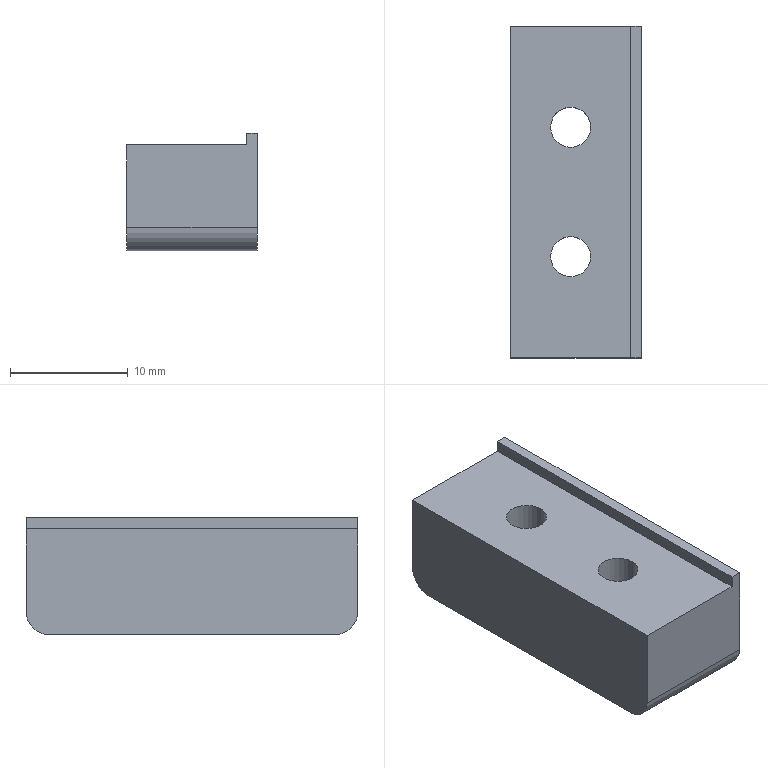Part | STEP file | 11-FG-SZ00911 | 1 solid | 20 faces | box 11.1 x 28.2 x 10 mm | volume 2496 mm3 | cylinder 10 | plane 10 | commonest cylinder face diameters 3.4 x4 6.5 x4 4 x2
STEP:
#1=CARTESIAN_POINT('',(3.25,5.5,3.4));
#2=VERTEX_POINT('',#1);
#3=CARTESIAN_POINT('',(-3.25,5.5,3.4));
#4=VERTEX_POINT('',#3);
#5=CARTESIAN_POINT('',(0.,5.5,3.4));
#6=DIRECTION('',(0.,0.,-1.));
#7=DIRECTION('',(-1.,0.,0.));
#8=AXIS2_PLACEMENT_3D('',#5,#6,#7);
#9=CIRCLE('',#8,3.25);
#10=EDGE_CURVE('',#2,#4,#9,.T.);
#11=ORIENTED_EDGE('',*,*,#10,.F.);
#12=CARTESIAN_POINT('',(3.25,5.5,0.));
#13=VERTEX_POINT('',#12);
#14=CARTESIAN_POINT('',(3.25,5.5,0.));
#15=DIRECTION('',(0.,0.,-1.));
#16=VECTOR('',#15,1000.);
#17=LINE('',#14,#16);
#18=EDGE_CURVE('',#2,#13,#17,.T.);
#19=ORIENTED_EDGE('',*,*,#18,.T.);
#20=CARTESIAN_POINT('',(-3.25,5.5,0.));
#21=VERTEX_POINT('',#20);
#22=CARTESIAN_POINT('',(0.,5.5,0.));
#23=DIRECTION('',(0.,0.,-1.));
#24=DIRECTION('',(-1.,0.,0.));
#25=AXIS2_PLACEMENT_3D('',#22,#23,#24);
#26=CIRCLE('',#25,3.25);
#27=EDGE_CURVE('',#13,#21,#26,.T.);
#28=ORIENTED_EDGE('',*,*,#27,.T.);
#29=CARTESIAN_POINT('',(-3.25,5.5,0.));
#30=DIRECTION('',(0.,0.,-1.));
#31=VECTOR('',#30,1000.);
#32=LINE('',#29,#31);
#33=EDGE_CURVE('',#4,#21,#32,.T.);
#34=ORIENTED_EDGE('',*,*,#33,.F.);
#35=EDGE_LOOP('',(#11,#19,#28,#34));
#36=FACE_OUTER_BOUND('',#35,.T.);
#37=CARTESIAN_POINT('',(0.,5.5,0.));
#38=DIRECTION('',(0.,0.,-1.));
#39=DIRECTION('',(-1.,0.,0.));
#40=AXIS2_PLACEMENT_3D('',#37,#38,#39);
#41=CYLINDRICAL_SURFACE('',#40,3.25);
#42=ADVANCED_FACE('',(#36),#41,.F.);
#43=CARTESIAN_POINT('',(1.7,5.5,9.));
#44=VERTEX_POINT('',#43);
#45=CARTESIAN_POINT('',(-1.7,5.5,9.));
#46=VERTEX_POINT('',#45);
#47=CARTESIAN_POINT('',(0.,5.5,9.));
#48=DIRECTION('',(0.,0.,-1.));
#49=DIRECTION('',(-1.,0.,0.));
#50=AXIS2_PLACEMENT_3D('',#47,#48,#49);
#51=CIRCLE('',#50,1.7);
#52=EDGE_CURVE('',#44,#46,#51,.T.);
#53=ORIENTED_EDGE('',*,*,#52,.F.);
#54=CARTESIAN_POINT('',(1.7,5.5,3.4));
#55=VERTEX_POINT('',#54);
#56=CARTESIAN_POINT('',(1.7,5.5,0.));
#57=DIRECTION('',(0.,0.,-1.));
#58=VECTOR('',#57,1000.);
#59=LINE('',#56,#58);
#60=EDGE_CURVE('',#44,#55,#59,.T.);
#61=ORIENTED_EDGE('',*,*,#60,.T.);
#62=CARTESIAN_POINT('',(-1.7,5.5,3.4));
#63=VERTEX_POINT('',#62);
#64=CARTESIAN_POINT('',(0.,5.5,3.4));
#65=DIRECTION('',(0.,0.,-1.));
#66=DIRECTION('',(-1.,0.,0.));
#67=AXIS2_PLACEMENT_3D('',#64,#65,#66);
#68=CIRCLE('',#67,1.7);
#69=EDGE_CURVE('',#55,#63,#68,.T.);
#70=ORIENTED_EDGE('',*,*,#69,.T.);
#71=CARTESIAN_POINT('',(-1.7,5.5,0.));
#72=DIRECTION('',(0.,0.,-1.));
#73=VECTOR('',#72,1000.);
#74=LINE('',#71,#73);
#75=EDGE_CURVE('',#46,#63,#74,.T.);
#76=ORIENTED_EDGE('',*,*,#75,.F.);
#77=EDGE_LOOP('',(#53,#61,#70,#76));
#78=FACE_OUTER_BOUND('',#77,.T.);
#79=CARTESIAN_POINT('',(0.,5.5,0.));
#80=DIRECTION('',(0.,0.,-1.));
#81=DIRECTION('',(-1.,0.,0.));
#82=AXIS2_PLACEMENT_3D('',#79,#80,#81);
#83=CYLINDRICAL_SURFACE('',#82,1.7);
#84=ADVANCED_FACE('',(#78),#83,.F.);
#85=CARTESIAN_POINT('',(3.25,-5.5,3.4));
#86=VERTEX_POINT('',#85);
#87=CARTESIAN_POINT('',(-3.25,-5.5,3.4));
#88=VERTEX_POINT('',#87);
#89=CARTESIAN_POINT('',(0.,-5.5,3.4));
#90=DIRECTION('',(0.,0.,-1.));
#91=DIRECTION('',(-1.,0.,0.));
#92=AXIS2_PLACEMENT_3D('',#89,#90,#91);
#93=CIRCLE('',#92,3.25);
#94=EDGE_CURVE('',#86,#88,#93,.T.);
#95=ORIENTED_EDGE('',*,*,#94,.F.);
#96=CARTESIAN_POINT('',(3.25,-5.5,0.));
#97=VERTEX_POINT('',#96);
#98=CARTESIAN_POINT('',(3.25,-5.5,0.));
#99=DIRECTION('',(0.,0.,-1.));
#100=VECTOR('',#99,1000.);
#101=LINE('',#98,#100);
#102=EDGE_CURVE('',#86,#97,#101,.T.);
#103=ORIENTED_EDGE('',*,*,#102,.T.);
#104=CARTESIAN_POINT('',(-3.25,-5.5,0.));
#105=VERTEX_POINT('',#104);
#106=CARTESIAN_POINT('',(0.,-5.5,0.));
#107=DIRECTION('',(0.,0.,-1.));
#108=DIRECTION('',(-1.,0.,0.));
#109=AXIS2_PLACEMENT_3D('',#106,#107,#108);
#110=CIRCLE('',#109,3.25);
#111=EDGE_CURVE('',#97,#105,#110,.T.);
#112=ORIENTED_EDGE('',*,*,#111,.T.);
#113=CARTESIAN_POINT('',(-3.25,-5.5,0.));
#114=DIRECTION('',(0.,0.,-1.));
#115=VECTOR('',#114,1000.);
#116=LINE('',#113,#115);
#117=EDGE_CURVE('',#88,#105,#116,.T.);
#118=ORIENTED_EDGE('',*,*,#117,.F.);
#119=EDGE_LOOP('',(#95,#103,#112,#118));
#120=FACE_OUTER_BOUND('',#119,.T.);
#121=CARTESIAN_POINT('',(0.,-5.5,0.));
#122=DIRECTION('',(0.,0.,-1.));
#123=DIRECTION('',(-1.,0.,0.));
#124=AXIS2_PLACEMENT_3D('',#121,#122,#123);
#125=CYLINDRICAL_SURFACE('',#124,3.25);
#126=ADVANCED_FACE('',(#120),#125,.F.);
#127=CARTESIAN_POINT('',(1.7,-5.5,9.));
#128=VERTEX_POINT('',#127);
#129=CARTESIAN_POINT('',(-1.7,-5.5,9.));
#130=VERTEX_POINT('',#129);
#131=CARTESIAN_POINT('',(0.,-5.5,9.));
#132=DIRECTION('',(0.,0.,-1.));
#133=DIRECTION('',(-1.,0.,0.));
#134=AXIS2_PLACEMENT_3D('',#131,#132,#133);
#135=CIRCLE('',#134,1.7);
#136=EDGE_CURVE('',#128,#130,#135,.T.);
#137=ORIENTED_EDGE('',*,*,#136,.F.);
#138=CARTESIAN_POINT('',(1.7,-5.5,3.4));
#139=VERTEX_POINT('',#138);
#140=CARTESIAN_POINT('',(1.7,-5.5,0.));
#141=DIRECTION('',(0.,0.,-1.));
#142=VECTOR('',#141,1000.);
#143=LINE('',#140,#142);
#144=EDGE_CURVE('',#128,#139,#143,.T.);
#145=ORIENTED_EDGE('',*,*,#144,.T.);
#146=CARTESIAN_POINT('',(-1.7,-5.5,3.4));
#147=VERTEX_POINT('',#146);
#148=CARTESIAN_POINT('',(0.,-5.5,3.4));
#149=DIRECTION('',(0.,0.,-1.));
#150=DIRECTION('',(-1.,0.,0.));
#151=AXIS2_PLACEMENT_3D('',#148,#149,#150);
#152=CIRCLE('',#151,1.7);
#153=EDGE_CURVE('',#139,#147,#152,.T.);
#154=ORIENTED_EDGE('',*,*,#153,.T.);
#155=CARTESIAN_POINT('',(-1.7,-5.5,0.));
#156=DIRECTION('',(0.,0.,-1.));
#157=VECTOR('',#156,1000.);
#158=LINE('',#155,#157);
#159=EDGE_CURVE('',#130,#147,#158,.T.);
#160=ORIENTED_EDGE('',*,*,#159,.F.);
#161=EDGE_LOOP('',(#137,#145,#154,#160));
#162=FACE_OUTER_BOUND('',#161,.T.);
#163=CARTESIAN_POINT('',(0.,-5.5,0.));
#164=DIRECTION('',(0.,0.,-1.));
#165=DIRECTION('',(-1.,0.,0.));
#166=AXIS2_PLACEMENT_3D('',#163,#164,#165);
#167=CYLINDRICAL_SURFACE('',#166,1.7);
#168=ADVANCED_FACE('',(#162),#167,.F.);
#169=CARTESIAN_POINT('',(5.1,-14.1,10.));
#170=VERTEX_POINT('',#169);
#171=CARTESIAN_POINT('',(5.1,14.1,10.));
#172=VERTEX_POINT('',#171);
#173=CARTESIAN_POINT('',(5.1,-14.1,10.));
#174=DIRECTION('',(0.,1.,0.));
#175=VECTOR('',#174,1000.);
#176=LINE('',#173,#175);
#177=EDGE_CURVE('',#170,#172,#176,.T.);
#178=ORIENTED_EDGE('',*,*,#177,.F.);
#179=CARTESIAN_POINT('',(6.,-14.1,10.));
#180=VERTEX_POINT('',#179);
#181=CARTESIAN_POINT('',(-6.,-14.1,10.));
#182=DIRECTION('',(1.,0.,0.));
#183=VECTOR('',#182,1000.);
#184=LINE('',#181,#183);
#185=EDGE_CURVE('',#170,#180,#184,.T.);
#186=ORIENTED_EDGE('',*,*,#185,.T.);
#187=CARTESIAN_POINT('',(6.,14.1,10.));
#188=VERTEX_POINT('',#187);
#189=CARTESIAN_POINT('',(6.,14.1,10.));
#190=DIRECTION('',(0.,1.,0.));
#191=VECTOR('',#190,1000.);
#192=LINE('',#189,#191);
#193=EDGE_CURVE('',#180,#188,#192,.T.);
#194=ORIENTED_EDGE('',*,*,#193,.T.);
#195=CARTESIAN_POINT('',(-6.,14.1,10.));
#196=DIRECTION('',(-1.,0.,0.));
#197=VECTOR('',#196,1000.);
#198=LINE('',#195,#197);
#199=EDGE_CURVE('',#188,#172,#198,.T.);
#200=ORIENTED_EDGE('',*,*,#199,.T.);
#201=EDGE_LOOP('',(#178,#186,#194,#200));
#202=FACE_OUTER_BOUND('',#201,.T.);
#203=CARTESIAN_POINT('',(0.,0.,10.));
#204=DIRECTION('',(0.,0.,1.));
#205=DIRECTION('',(1.,0.,0.));
#206=AXIS2_PLACEMENT_3D('',#203,#204,#205);
#207=PLANE('',#206);
#208=ADVANCED_FACE('',(#202),#207,.T.);
#209=CARTESIAN_POINT('',(6.,-12.1,0.));
#210=VERTEX_POINT('',#209);
#211=CARTESIAN_POINT('',(6.,12.1,0.));
#212=VERTEX_POINT('',#211);
#213=CARTESIAN_POINT('',(6.,14.1,0.));
#214=DIRECTION('',(0.,1.,0.));
#215=VECTOR('',#214,1000.);
#216=LINE('',#213,#215);
#217=EDGE_CURVE('',#210,#212,#216,.T.);
#218=ORIENTED_EDGE('',*,*,#217,.T.);
#219=CARTESIAN_POINT('',(6.,14.1,2.));
#220=VERTEX_POINT('',#219);
#221=CARTESIAN_POINT('',(6.,12.1,2.));
#222=DIRECTION('',(1.,0.,0.));
#223=DIRECTION('',(0.,-1.,0.));
#224=AXIS2_PLACEMENT_3D('',#221,#222,#223);
#225=CIRCLE('',#224,2.);
#226=EDGE_CURVE('',#212,#220,#225,.T.);
#227=ORIENTED_EDGE('',*,*,#226,.T.);
#228=CARTESIAN_POINT('',(6.,14.1,10.));
#229=DIRECTION('',(0.,0.,-1.));
#230=VECTOR('',#229,1000.);
#231=LINE('',#228,#230);
#232=EDGE_CURVE('',#188,#220,#231,.T.);
#233=ORIENTED_EDGE('',*,*,#232,.F.);
#234=ORIENTED_EDGE('',*,*,#193,.F.);
#235=CARTESIAN_POINT('',(6.,-14.1,2.));
#236=VERTEX_POINT('',#235);
#237=CARTESIAN_POINT('',(6.,-14.1,10.));
#238=DIRECTION('',(0.,0.,-1.));
#239=VECTOR('',#238,1000.);
#240=LINE('',#237,#239);
#241=EDGE_CURVE('',#180,#236,#240,.T.);
#242=ORIENTED_EDGE('',*,*,#241,.T.);
#243=CARTESIAN_POINT('',(6.,-12.1,2.));
#244=DIRECTION('',(1.,0.,0.));
#245=DIRECTION('',(0.,-1.,0.));
#246=AXIS2_PLACEMENT_3D('',#243,#244,#245);
#247=CIRCLE('',#246,2.);
#248=EDGE_CURVE('',#236,#210,#247,.T.);
#249=ORIENTED_EDGE('',*,*,#248,.T.);
#250=EDGE_LOOP('',(#218,#227,#233,#234,#242,#249));
#251=FACE_OUTER_BOUND('',#250,.T.);
#252=CARTESIAN_POINT('',(6.,14.1,10.));
#253=DIRECTION('',(-1.,0.,0.));
#254=DIRECTION('',(0.,-1.,0.));
#255=AXIS2_PLACEMENT_3D('',#252,#253,#254);
#256=PLANE('',#255);
#257=ADVANCED_FACE('',(#251),#256,.F.);
#258=CARTESIAN_POINT('',(-5.1,14.1,2.));
#259=VERTEX_POINT('',#258);
#260=CARTESIAN_POINT('',(-6.,14.1,2.));
#261=DIRECTION('',(-1.,0.,0.));
#262=VECTOR('',#261,1000.);
#263=LINE('',#260,#262);
#264=EDGE_CURVE('',#220,#259,#263,.T.);
#265=ORIENTED_EDGE('',*,*,#264,.T.);
#266=CARTESIAN_POINT('',(-5.1,14.1,9.));
#267=VERTEX_POINT('',#266);
#268=CARTESIAN_POINT('',(-5.1,14.1,10.));
#269=DIRECTION('',(0.,0.,-1.));
#270=VECTOR('',#269,1000.);
#271=LINE('',#268,#270);
#272=EDGE_CURVE('',#267,#259,#271,.T.);
#273=ORIENTED_EDGE('',*,*,#272,.F.);
#274=CARTESIAN_POINT('',(5.1,14.1,9.));
#275=VERTEX_POINT('',#274);
#276=CARTESIAN_POINT('',(5.1,14.1,9.));
#277=DIRECTION('',(-1.,0.,0.));
#278=VECTOR('',#277,1000.);
#279=LINE('',#276,#278);
#280=EDGE_CURVE('',#275,#267,#279,.T.);
#281=ORIENTED_EDGE('',*,*,#280,.F.);
#282=CARTESIAN_POINT('',(5.1,14.1,9.));
#283=DIRECTION('',(0.,0.,-1.));
#284=VECTOR('',#283,1000.);
#285=LINE('',#282,#284);
#286=EDGE_CURVE('',#172,#275,#285,.T.);
#287=ORIENTED_EDGE('',*,*,#286,.F.);
#288=ORIENTED_EDGE('',*,*,#199,.F.);
#289=ORIENTED_EDGE('',*,*,#232,.T.);
#290=EDGE_LOOP('',(#265,#273,#281,#287,#288,#289));
#291=FACE_OUTER_BOUND('',#290,.T.);
#292=CARTESIAN_POINT('',(-6.,14.1,10.));
#293=DIRECTION('',(0.,-1.,0.));
#294=DIRECTION('',(0.,0.,-1.));
#295=AXIS2_PLACEMENT_3D('',#292,#293,#294);
#296=PLANE('',#295);
#297=ADVANCED_FACE('',(#291),#296,.F.);
#298=CARTESIAN_POINT('',(5.1,-14.1,9.));
#299=VERTEX_POINT('',#298);
#300=CARTESIAN_POINT('',(-5.1,-14.1,9.));
#301=VERTEX_POINT('',#300);
#302=CARTESIAN_POINT('',(5.1,-14.1,9.));
#303=DIRECTION('',(-1.,0.,0.));
#304=VECTOR('',#303,1000.);
#305=LINE('',#302,#304);
#306=EDGE_CURVE('',#299,#301,#305,.T.);
#307=ORIENTED_EDGE('',*,*,#306,.T.);
#308=CARTESIAN_POINT('',(-5.1,-14.1,2.));
#309=VERTEX_POINT('',#308);
#310=CARTESIAN_POINT('',(-5.1,-14.1,10.));
#311=DIRECTION('',(0.,0.,-1.));
#312=VECTOR('',#311,1000.);
#313=LINE('',#310,#312);
#314=EDGE_CURVE('',#301,#309,#313,.T.);
#315=ORIENTED_EDGE('',*,*,#314,.T.);
#316=CARTESIAN_POINT('',(-6.,-14.1,2.));
#317=DIRECTION('',(1.,0.,0.));
#318=VECTOR('',#317,1000.);
#319=LINE('',#316,#318);
#320=EDGE_CURVE('',#309,#236,#319,.T.);
#321=ORIENTED_EDGE('',*,*,#320,.T.);
#322=ORIENTED_EDGE('',*,*,#241,.F.);
#323=ORIENTED_EDGE('',*,*,#185,.F.);
#324=CARTESIAN_POINT('',(5.1,-14.1,9.));
#325=DIRECTION('',(0.,0.,-1.));
#326=VECTOR('',#325,1000.);
#327=LINE('',#324,#326);
#328=EDGE_CURVE('',#170,#299,#327,.T.);
#329=ORIENTED_EDGE('',*,*,#328,.T.);
#330=EDGE_LOOP('',(#307,#315,#321,#322,#323,#329));
#331=FACE_OUTER_BOUND('',#330,.T.);
#332=CARTESIAN_POINT('',(-6.,-14.1,10.));
#333=DIRECTION('',(0.,1.,0.));
#334=DIRECTION('',(0.,0.,1.));
#335=AXIS2_PLACEMENT_3D('',#332,#333,#334);
#336=PLANE('',#335);
#337=ADVANCED_FACE('',(#331),#336,.F.);
#338=CARTESIAN_POINT('',(0.,5.5,0.));
#339=DIRECTION('',(0.,0.,-1.));
#340=DIRECTION('',(-1.,0.,0.));
#341=AXIS2_PLACEMENT_3D('',#338,#339,#340);
#342=CIRCLE('',#341,3.25);
#343=EDGE_CURVE('',#21,#13,#342,.T.);
#344=ORIENTED_EDGE('',*,*,#343,.F.);
#345=ORIENTED_EDGE('',*,*,#27,.F.);
#346=EDGE_LOOP('',(#344,#345));
#347=FACE_BOUND('',#346,.T.);
#348=CARTESIAN_POINT('',(0.,-5.5,0.));
#349=DIRECTION('',(0.,0.,-1.));
#350=DIRECTION('',(-1.,0.,0.));
#351=AXIS2_PLACEMENT_3D('',#348,#349,#350);
#352=CIRCLE('',#351,3.25);
#353=EDGE_CURVE('',#105,#97,#352,.T.);
#354=ORIENTED_EDGE('',*,*,#353,.F.);
#355=ORIENTED_EDGE('',*,*,#111,.F.);
#356=EDGE_LOOP('',(#354,#355));
#357=FACE_BOUND('',#356,.T.);
#358=CARTESIAN_POINT('',(-5.1,-12.1,0.));
#359=VERTEX_POINT('',#358);
#360=CARTESIAN_POINT('',(0.,-12.1,0.));
#361=DIRECTION('',(-1.,0.,0.));
#362=VECTOR('',#361,1000.);
#363=LINE('',#360,#362);
#364=EDGE_CURVE('',#210,#359,#363,.T.);
#365=ORIENTED_EDGE('',*,*,#364,.T.);
#366=CARTESIAN_POINT('',(-5.1,12.1,0.));
#367=VERTEX_POINT('',#366);
#368=CARTESIAN_POINT('',(-5.1,-14.1,0.));
#369=DIRECTION('',(0.,1.,0.));
#370=VECTOR('',#369,1000.);
#371=LINE('',#368,#370);
#372=EDGE_CURVE('',#359,#367,#371,.T.);
#373=ORIENTED_EDGE('',*,*,#372,.T.);
#374=CARTESIAN_POINT('',(0.,12.1,0.));
#375=DIRECTION('',(1.,0.,0.));
#376=VECTOR('',#375,1000.);
#377=LINE('',#374,#376);
#378=EDGE_CURVE('',#367,#212,#377,.T.);
#379=ORIENTED_EDGE('',*,*,#378,.T.);
#380=ORIENTED_EDGE('',*,*,#217,.F.);
#381=EDGE_LOOP('',(#365,#373,#379,#380));
#382=FACE_OUTER_BOUND('',#381,.T.);
#383=CARTESIAN_POINT('',(0.,0.,0.));
#384=DIRECTION('',(0.,0.,1.));
#385=DIRECTION('',(1.,0.,0.));
#386=AXIS2_PLACEMENT_3D('',#383,#384,#385);
#387=PLANE('',#386);
#388=ADVANCED_FACE('',(#347,#357,#382),#387,.F.);
#389=ORIENTED_EDGE('',*,*,#286,.T.);
#390=CARTESIAN_POINT('',(5.1,-14.1,9.));
#391=DIRECTION('',(0.,1.,0.));
#392=VECTOR('',#391,1000.);
#393=LINE('',#390,#392);
#394=EDGE_CURVE('',#299,#275,#393,.T.);
#395=ORIENTED_EDGE('',*,*,#394,.F.);
#396=ORIENTED_EDGE('',*,*,#328,.F.);
#397=ORIENTED_EDGE('',*,*,#177,.T.);
#398=EDGE_LOOP('',(#389,#395,#396,#397));
#399=FACE_OUTER_BOUND('',#398,.T.);
#400=CARTESIAN_POINT('',(5.1,-14.1,9.));
#401=DIRECTION('',(1.,0.,0.));
#402=DIRECTION('',(0.,0.,-1.));
#403=AXIS2_PLACEMENT_3D('',#400,#401,#402);
#404=PLANE('',#403);
#405=ADVANCED_FACE('',(#399),#404,.F.);
#406=CARTESIAN_POINT('',(0.,5.5,9.));
#407=DIRECTION('',(0.,0.,-1.));
#408=DIRECTION('',(-1.,0.,0.));
#409=AXIS2_PLACEMENT_3D('',#406,#407,#408);
#410=CIRCLE('',#409,1.7);
#411=EDGE_CURVE('',#46,#44,#410,.T.);
#412=ORIENTED_EDGE('',*,*,#411,.T.);
#413=ORIENTED_EDGE('',*,*,#52,.T.);
#414=EDGE_LOOP('',(#412,#413));
#415=FACE_BOUND('',#414,.T.);
#416=CARTESIAN_POINT('',(0.,-5.5,9.));
#417=DIRECTION('',(0.,0.,-1.));
#418=DIRECTION('',(-1.,0.,0.));
#419=AXIS2_PLACEMENT_3D('',#416,#417,#418);
#420=CIRCLE('',#419,1.7);
#421=EDGE_CURVE('',#130,#128,#420,.T.);
#422=ORIENTED_EDGE('',*,*,#421,.T.);
#423=ORIENTED_EDGE('',*,*,#136,.T.);
#424=EDGE_LOOP('',(#422,#423));
#425=FACE_BOUND('',#424,.T.);
#426=ORIENTED_EDGE('',*,*,#280,.T.);
#427=CARTESIAN_POINT('',(-5.1,-14.1,9.));
#428=DIRECTION('',(0.,1.,0.));
#429=VECTOR('',#428,1000.);
#430=LINE('',#427,#429);
#431=EDGE_CURVE('',#301,#267,#430,.T.);
#432=ORIENTED_EDGE('',*,*,#431,.F.);
#433=ORIENTED_EDGE('',*,*,#306,.F.);
#434=ORIENTED_EDGE('',*,*,#394,.T.);
#435=EDGE_LOOP('',(#426,#432,#433,#434));
#436=FACE_OUTER_BOUND('',#435,.T.);
#437=CARTESIAN_POINT('',(5.1,-14.1,9.));
#438=DIRECTION('',(0.,0.,-1.));
#439=DIRECTION('',(-1.,0.,0.));
#440=AXIS2_PLACEMENT_3D('',#437,#438,#439);
#441=PLANE('',#440);
#442=ADVANCED_FACE('',(#415,#425,#436),#441,.F.);
#443=ORIENTED_EDGE('',*,*,#144,.F.);
#444=ORIENTED_EDGE('',*,*,#421,.F.);
#445=ORIENTED_EDGE('',*,*,#159,.T.);
#446=CARTESIAN_POINT('',(0.,-5.5,3.4));
#447=DIRECTION('',(0.,0.,-1.));
#448=DIRECTION('',(-1.,0.,0.));
#449=AXIS2_PLACEMENT_3D('',#446,#447,#448);
#450=CIRCLE('',#449,1.7);
#451=EDGE_CURVE('',#147,#139,#450,.T.);
#452=ORIENTED_EDGE('',*,*,#451,.T.);
#453=EDGE_LOOP('',(#443,#444,#445,#452));
#454=FACE_OUTER_BOUND('',#453,.T.);
#455=CARTESIAN_POINT('',(0.,-5.5,0.));
#456=DIRECTION('',(0.,0.,-1.));
#457=DIRECTION('',(-1.,0.,0.));
#458=AXIS2_PLACEMENT_3D('',#455,#456,#457);
#459=CYLINDRICAL_SURFACE('',#458,1.7);
#460=ADVANCED_FACE('',(#454),#459,.F.);
#461=ORIENTED_EDGE('',*,*,#451,.F.);
#462=ORIENTED_EDGE('',*,*,#153,.F.);
#463=EDGE_LOOP('',(#461,#462));
#464=FACE_BOUND('',#463,.T.);
#465=CARTESIAN_POINT('',(0.,-5.5,3.4));
#466=DIRECTION('',(0.,0.,-1.));
#467=DIRECTION('',(-1.,0.,0.));
#468=AXIS2_PLACEMENT_3D('',#465,#466,#467);
#469=CIRCLE('',#468,3.25);
#470=EDGE_CURVE('',#88,#86,#469,.T.);
#471=ORIENTED_EDGE('',*,*,#470,.T.);
#472=ORIENTED_EDGE('',*,*,#94,.T.);
#473=EDGE_LOOP('',(#471,#472));
#474=FACE_OUTER_BOUND('',#473,.T.);
#475=CARTESIAN_POINT('',(1.7,-5.5,3.4));
#476=DIRECTION('',(0.,0.,1.));
#477=DIRECTION('',(1.,0.,0.));
#478=AXIS2_PLACEMENT_3D('',#475,#476,#477);
#479=PLANE('',#478);
#480=ADVANCED_FACE('',(#464,#474),#479,.F.);
#481=ORIENTED_EDGE('',*,*,#102,.F.);
#482=ORIENTED_EDGE('',*,*,#470,.F.);
#483=ORIENTED_EDGE('',*,*,#117,.T.);
#484=ORIENTED_EDGE('',*,*,#353,.T.);
#485=EDGE_LOOP('',(#481,#482,#483,#484));
#486=FACE_OUTER_BOUND('',#485,.T.);
#487=CARTESIAN_POINT('',(0.,-5.5,0.));
#488=DIRECTION('',(0.,0.,-1.));
#489=DIRECTION('',(-1.,0.,0.));
#490=AXIS2_PLACEMENT_3D('',#487,#488,#489);
#491=CYLINDRICAL_SURFACE('',#490,3.25);
#492=ADVANCED_FACE('',(#486),#491,.F.);
#493=ORIENTED_EDGE('',*,*,#60,.F.);
#494=ORIENTED_EDGE('',*,*,#411,.F.);
#495=ORIENTED_EDGE('',*,*,#75,.T.);
#496=CARTESIAN_POINT('',(0.,5.5,3.4));
#497=DIRECTION('',(0.,0.,-1.));
#498=DIRECTION('',(-1.,0.,0.));
#499=AXIS2_PLACEMENT_3D('',#496,#497,#498);
#500=CIRCLE('',#499,1.7);
#501=EDGE_CURVE('',#63,#55,#500,.T.);
#502=ORIENTED_EDGE('',*,*,#501,.T.);
#503=EDGE_LOOP('',(#493,#494,#495,#502));
#504=FACE_OUTER_BOUND('',#503,.T.);
#505=CARTESIAN_POINT('',(0.,5.5,0.));
#506=DIRECTION('',(0.,0.,-1.));
#507=DIRECTION('',(-1.,0.,0.));
#508=AXIS2_PLACEMENT_3D('',#505,#506,#507);
#509=CYLINDRICAL_SURFACE('',#508,1.7);
#510=ADVANCED_FACE('',(#504),#509,.F.);
#511=ORIENTED_EDGE('',*,*,#501,.F.);
#512=ORIENTED_EDGE('',*,*,#69,.F.);
#513=EDGE_LOOP('',(#511,#512));
#514=FACE_BOUND('',#513,.T.);
#515=CARTESIAN_POINT('',(0.,5.5,3.4));
#516=DIRECTION('',(0.,0.,-1.));
#517=DIRECTION('',(-1.,0.,0.));
#518=AXIS2_PLACEMENT_3D('',#515,#516,#517);
#519=CIRCLE('',#518,3.25);
#520=EDGE_CURVE('',#4,#2,#519,.T.);
#521=ORIENTED_EDGE('',*,*,#520,.T.);
#522=ORIENTED_EDGE('',*,*,#10,.T.);
#523=EDGE_LOOP('',(#521,#522));
#524=FACE_OUTER_BOUND('',#523,.T.);
#525=CARTESIAN_POINT('',(1.7,5.5,3.4));
#526=DIRECTION('',(0.,0.,1.));
#527=DIRECTION('',(1.,0.,0.));
#528=AXIS2_PLACEMENT_3D('',#525,#526,#527);
#529=PLANE('',#528);
#530=ADVANCED_FACE('',(#514,#524),#529,.F.);
#531=ORIENTED_EDGE('',*,*,#18,.F.);
#532=ORIENTED_EDGE('',*,*,#520,.F.);
#533=ORIENTED_EDGE('',*,*,#33,.T.);
#534=ORIENTED_EDGE('',*,*,#343,.T.);
#535=EDGE_LOOP('',(#531,#532,#533,#534));
#536=FACE_OUTER_BOUND('',#535,.T.);
#537=CARTESIAN_POINT('',(0.,5.5,0.));
#538=DIRECTION('',(0.,0.,-1.));
#539=DIRECTION('',(-1.,0.,0.));
#540=AXIS2_PLACEMENT_3D('',#537,#538,#539);
#541=CYLINDRICAL_SURFACE('',#540,3.25);
#542=ADVANCED_FACE('',(#536),#541,.F.);
#543=CARTESIAN_POINT('',(-5.1,12.1,2.));
#544=DIRECTION('',(-1.,0.,0.));
#545=DIRECTION('',(0.,0.,-1.));
#546=AXIS2_PLACEMENT_3D('',#543,#544,#545);
#547=CIRCLE('',#546,2.);
#548=EDGE_CURVE('',#259,#367,#547,.T.);
#549=ORIENTED_EDGE('',*,*,#548,.F.);
#550=ORIENTED_EDGE('',*,*,#264,.F.);
#551=ORIENTED_EDGE('',*,*,#226,.F.);
#552=ORIENTED_EDGE('',*,*,#378,.F.);
#553=EDGE_LOOP('',(#549,#550,#551,#552));
#554=FACE_OUTER_BOUND('',#553,.T.);
#555=CARTESIAN_POINT('',(-6.,12.1,2.));
#556=DIRECTION('',(-1.,0.,0.));
#557=DIRECTION('',(0.,0.,1.));
#558=AXIS2_PLACEMENT_3D('',#555,#556,#557);
#559=CYLINDRICAL_SURFACE('',#558,2.);
#560=ADVANCED_FACE('',(#554),#559,.T.);
#561=CARTESIAN_POINT('',(-5.1,-12.1,2.));
#562=DIRECTION('',(-1.,0.,0.));
#563=DIRECTION('',(0.,0.,-1.));
#564=AXIS2_PLACEMENT_3D('',#561,#562,#563);
#565=CIRCLE('',#564,2.);
#566=EDGE_CURVE('',#359,#309,#565,.T.);
#567=ORIENTED_EDGE('',*,*,#566,.F.);
#568=ORIENTED_EDGE('',*,*,#364,.F.);
#569=ORIENTED_EDGE('',*,*,#248,.F.);
#570=ORIENTED_EDGE('',*,*,#320,.F.);
#571=EDGE_LOOP('',(#567,#568,#569,#570));
#572=FACE_OUTER_BOUND('',#571,.T.);
#573=CARTESIAN_POINT('',(-6.,-12.1,2.));
#574=DIRECTION('',(1.,0.,0.));
#575=DIRECTION('',(0.,0.,-1.));
#576=AXIS2_PLACEMENT_3D('',#573,#574,#575);
#577=CYLINDRICAL_SURFACE('',#576,2.);
#578=ADVANCED_FACE('',(#572),#577,.T.);
#579=ORIENTED_EDGE('',*,*,#272,.T.);
#580=ORIENTED_EDGE('',*,*,#548,.T.);
#581=ORIENTED_EDGE('',*,*,#372,.F.);
#582=ORIENTED_EDGE('',*,*,#566,.T.);
#583=ORIENTED_EDGE('',*,*,#314,.F.);
#584=ORIENTED_EDGE('',*,*,#431,.T.);
#585=EDGE_LOOP('',(#579,#580,#581,#582,#583,#584));
#586=FACE_OUTER_BOUND('',#585,.T.);
#587=CARTESIAN_POINT('',(-5.1,-14.1,10.));
#588=DIRECTION('',(1.,0.,0.));
#589=DIRECTION('',(0.,0.,-1.));
#590=AXIS2_PLACEMENT_3D('',#587,#588,#589);
#591=PLANE('',#590);
#592=ADVANCED_FACE('',(#586),#591,.F.);
#593=CLOSED_SHELL('',(#42,#84,#126,#168,#208,#257,#297,#337,#388,#405,#442,#460,#480,#492,#510,#530,#542,#560,#578,#592));
#594=MANIFOLD_SOLID_BREP('',#593);
#595=CARTESIAN_POINT('',(0.,0.,0.));
#596=DIRECTION('',(0.,0.,1.));
#597=DIRECTION('',(1.,0.,0.));
#598=AXIS2_PLACEMENT_3D('',#595,#596,#597);
#599=(LENGTH_UNIT()NAMED_UNIT(*)SI_UNIT(.MILLI.,.METRE.));
#600=UNCERTAINTY_MEASURE_WITH_UNIT(LENGTH_MEASURE(0.00001),#599,'','');
#601=(NAMED_UNIT(*)PLANE_ANGLE_UNIT()SI_UNIT($,.RADIAN.));
#602=(NAMED_UNIT(*)SI_UNIT($,.STERADIAN.)SOLID_ANGLE_UNIT());
#603=(GEOMETRIC_REPRESENTATION_CONTEXT(3)GLOBAL_UNCERTAINTY_ASSIGNED_CONTEXT((#600))GLOBAL_UNIT_ASSIGNED_CONTEXT((#599,#601,#602))REPRESENTATION_CONTEXT('',''));
#604=ADVANCED_BREP_SHAPE_REPRESENTATION('',(#594,#598),#603);